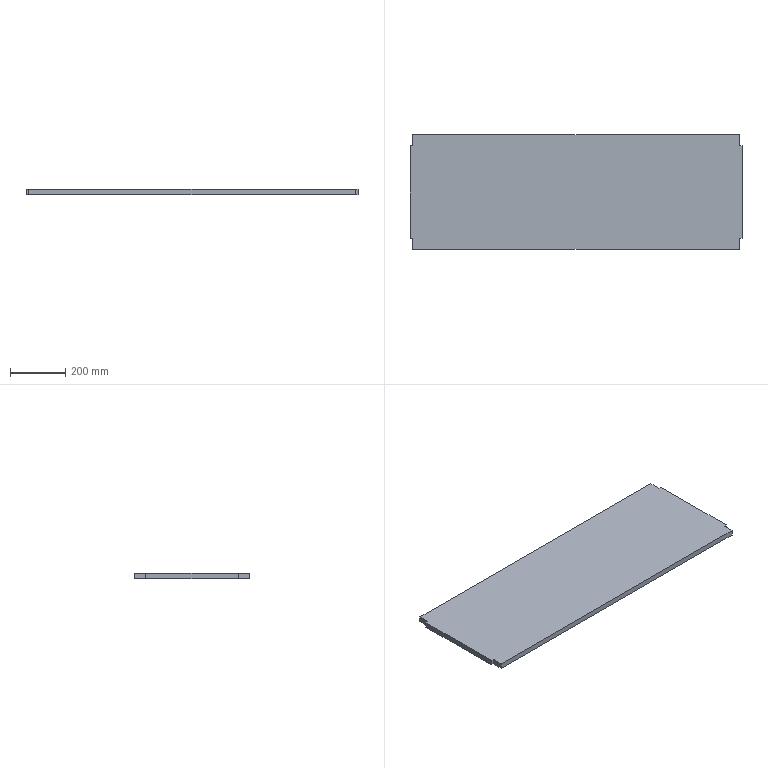Part | SolidWorks | features Extrusion 1, ICE 1 | 1 solid | 14 faces | box 1200 x 415 x 20 mm | volume 9928000 mm3 | plane 14
STEP:
#1=CARTESIAN_POINT('',(0.,375.,0.));
#2=VERTEX_POINT('',#1);
#3=CARTESIAN_POINT('',(0.,40.,0.));
#4=VERTEX_POINT('',#3);
#5=CARTESIAN_POINT('',(0.,0.,0.));
#6=DIRECTION('',(0.,-1.,0.));
#7=VECTOR('',#6,1000.);
#8=LINE('',#5,#7);
#9=EDGE_CURVE('',#2,#4,#8,.T.);
#10=ORIENTED_EDGE('',*,*,#9,.T.);
#11=CARTESIAN_POINT('',(0.,40.,20.));
#12=VERTEX_POINT('',#11);
#13=CARTESIAN_POINT('',(0.,40.,-260.));
#14=DIRECTION('',(0.,0.,1.));
#15=VECTOR('',#14,1000.);
#16=LINE('',#13,#15);
#17=EDGE_CURVE('',#4,#12,#16,.T.);
#18=ORIENTED_EDGE('',*,*,#17,.T.);
#19=CARTESIAN_POINT('',(0.,375.,20.));
#20=VERTEX_POINT('',#19);
#21=CARTESIAN_POINT('',(0.,0.,20.));
#22=DIRECTION('',(0.,-1.,0.));
#23=VECTOR('',#22,1000.);
#24=LINE('',#21,#23);
#25=EDGE_CURVE('',#20,#12,#24,.T.);
#26=ORIENTED_EDGE('',*,*,#25,.F.);
#27=CARTESIAN_POINT('',(0.,375.,-260.));
#28=DIRECTION('',(0.,0.,1.));
#29=VECTOR('',#28,1000.);
#30=LINE('',#27,#29);
#31=EDGE_CURVE('',#2,#20,#30,.T.);
#32=ORIENTED_EDGE('',*,*,#31,.F.);
#33=EDGE_LOOP('',(#10,#18,#26,#32));
#34=FACE_OUTER_BOUND('',#33,.T.);
#35=CARTESIAN_POINT('',(0.,0.,20.));
#36=DIRECTION('',(1.,0.,0.));
#37=DIRECTION('',(0.,0.,-1.));
#38=AXIS2_PLACEMENT_3D('',#35,#36,#37);
#39=PLANE('',#38);
#40=ADVANCED_FACE('',(#34),#39,.F.);
#41=CARTESIAN_POINT('',(10.,0.,20.));
#42=VERTEX_POINT('',#41);
#43=CARTESIAN_POINT('',(1190.,0.,20.));
#44=VERTEX_POINT('',#43);
#45=CARTESIAN_POINT('',(0.,0.,20.));
#46=DIRECTION('',(1.,0.,0.));
#47=VECTOR('',#46,1000.);
#48=LINE('',#45,#47);
#49=EDGE_CURVE('',#42,#44,#48,.T.);
#50=ORIENTED_EDGE('',*,*,#49,.F.);
#51=CARTESIAN_POINT('',(10.,0.,0.));
#52=VERTEX_POINT('',#51);
#53=CARTESIAN_POINT('',(10.,0.,-260.));
#54=DIRECTION('',(0.,0.,1.));
#55=VECTOR('',#54,1000.);
#56=LINE('',#53,#55);
#57=EDGE_CURVE('',#52,#42,#56,.T.);
#58=ORIENTED_EDGE('',*,*,#57,.F.);
#59=CARTESIAN_POINT('',(1190.,0.,0.));
#60=VERTEX_POINT('',#59);
#61=CARTESIAN_POINT('',(0.,0.,0.));
#62=DIRECTION('',(1.,0.,0.));
#63=VECTOR('',#62,1000.);
#64=LINE('',#61,#63);
#65=EDGE_CURVE('',#52,#60,#64,.T.);
#66=ORIENTED_EDGE('',*,*,#65,.T.);
#67=CARTESIAN_POINT('',(1190.,0.,-260.));
#68=DIRECTION('',(0.,0.,1.));
#69=VECTOR('',#68,1000.);
#70=LINE('',#67,#69);
#71=EDGE_CURVE('',#60,#44,#70,.T.);
#72=ORIENTED_EDGE('',*,*,#71,.T.);
#73=EDGE_LOOP('',(#50,#58,#66,#72));
#74=FACE_OUTER_BOUND('',#73,.T.);
#75=CARTESIAN_POINT('',(0.,0.,20.));
#76=DIRECTION('',(0.,1.,0.));
#77=DIRECTION('',(0.,0.,1.));
#78=AXIS2_PLACEMENT_3D('',#75,#76,#77);
#79=PLANE('',#78);
#80=ADVANCED_FACE('',(#74),#79,.F.);
#81=CARTESIAN_POINT('',(1200.,40.,20.));
#82=VERTEX_POINT('',#81);
#83=CARTESIAN_POINT('',(1200.,375.,20.));
#84=VERTEX_POINT('',#83);
#85=CARTESIAN_POINT('',(1200.,0.,20.));
#86=DIRECTION('',(0.,1.,0.));
#87=VECTOR('',#86,1000.);
#88=LINE('',#85,#87);
#89=EDGE_CURVE('',#82,#84,#88,.T.);
#90=ORIENTED_EDGE('',*,*,#89,.F.);
#91=CARTESIAN_POINT('',(1200.,40.,0.));
#92=VERTEX_POINT('',#91);
#93=CARTESIAN_POINT('',(1200.,40.,-260.));
#94=DIRECTION('',(0.,0.,1.));
#95=VECTOR('',#94,1000.);
#96=LINE('',#93,#95);
#97=EDGE_CURVE('',#92,#82,#96,.T.);
#98=ORIENTED_EDGE('',*,*,#97,.F.);
#99=CARTESIAN_POINT('',(1200.,375.,0.));
#100=VERTEX_POINT('',#99);
#101=CARTESIAN_POINT('',(1200.,0.,0.));
#102=DIRECTION('',(0.,1.,0.));
#103=VECTOR('',#102,1000.);
#104=LINE('',#101,#103);
#105=EDGE_CURVE('',#92,#100,#104,.T.);
#106=ORIENTED_EDGE('',*,*,#105,.T.);
#107=CARTESIAN_POINT('',(1200.,375.,-260.));
#108=DIRECTION('',(0.,0.,1.));
#109=VECTOR('',#108,1000.);
#110=LINE('',#107,#109);
#111=EDGE_CURVE('',#100,#84,#110,.T.);
#112=ORIENTED_EDGE('',*,*,#111,.T.);
#113=EDGE_LOOP('',(#90,#98,#106,#112));
#114=FACE_OUTER_BOUND('',#113,.T.);
#115=CARTESIAN_POINT('',(1200.,0.,20.));
#116=DIRECTION('',(-1.,0.,0.));
#117=DIRECTION('',(0.,0.,1.));
#118=AXIS2_PLACEMENT_3D('',#115,#116,#117);
#119=PLANE('',#118);
#120=ADVANCED_FACE('',(#114),#119,.F.);
#121=CARTESIAN_POINT('',(1190.,415.,20.));
#122=VERTEX_POINT('',#121);
#123=CARTESIAN_POINT('',(10.,415.,20.));
#124=VERTEX_POINT('',#123);
#125=CARTESIAN_POINT('',(0.,415.,20.));
#126=DIRECTION('',(-1.,0.,0.));
#127=VECTOR('',#126,1000.);
#128=LINE('',#125,#127);
#129=EDGE_CURVE('',#122,#124,#128,.T.);
#130=ORIENTED_EDGE('',*,*,#129,.F.);
#131=CARTESIAN_POINT('',(1190.,415.,0.));
#132=VERTEX_POINT('',#131);
#133=CARTESIAN_POINT('',(1190.,415.,-260.));
#134=DIRECTION('',(0.,0.,1.));
#135=VECTOR('',#134,1000.);
#136=LINE('',#133,#135);
#137=EDGE_CURVE('',#132,#122,#136,.T.);
#138=ORIENTED_EDGE('',*,*,#137,.F.);
#139=CARTESIAN_POINT('',(10.,415.,0.));
#140=VERTEX_POINT('',#139);
#141=CARTESIAN_POINT('',(0.,415.,0.));
#142=DIRECTION('',(-1.,0.,0.));
#143=VECTOR('',#142,1000.);
#144=LINE('',#141,#143);
#145=EDGE_CURVE('',#132,#140,#144,.T.);
#146=ORIENTED_EDGE('',*,*,#145,.T.);
#147=CARTESIAN_POINT('',(10.,415.,-260.));
#148=DIRECTION('',(0.,0.,1.));
#149=VECTOR('',#148,1000.);
#150=LINE('',#147,#149);
#151=EDGE_CURVE('',#140,#124,#150,.T.);
#152=ORIENTED_EDGE('',*,*,#151,.T.);
#153=EDGE_LOOP('',(#130,#138,#146,#152));
#154=FACE_OUTER_BOUND('',#153,.T.);
#155=CARTESIAN_POINT('',(0.,415.,20.));
#156=DIRECTION('',(0.,-1.,0.));
#157=DIRECTION('',(0.,0.,-1.));
#158=AXIS2_PLACEMENT_3D('',#155,#156,#157);
#159=PLANE('',#158);
#160=ADVANCED_FACE('',(#154),#159,.F.);
#161=ORIENTED_EDGE('',*,*,#25,.T.);
#162=CARTESIAN_POINT('',(10.,40.,20.));
#163=VERTEX_POINT('',#162);
#164=CARTESIAN_POINT('',(0.,40.,20.));
#165=DIRECTION('',(-1.,0.,0.));
#166=VECTOR('',#165,1000.);
#167=LINE('',#164,#166);
#168=EDGE_CURVE('',#163,#12,#167,.T.);
#169=ORIENTED_EDGE('',*,*,#168,.F.);
#170=CARTESIAN_POINT('',(10.,0.,20.));
#171=DIRECTION('',(0.,1.,0.));
#172=VECTOR('',#171,1000.);
#173=LINE('',#170,#172);
#174=EDGE_CURVE('',#42,#163,#173,.T.);
#175=ORIENTED_EDGE('',*,*,#174,.F.);
#176=ORIENTED_EDGE('',*,*,#49,.T.);
#177=CARTESIAN_POINT('',(1190.,40.,20.));
#178=VERTEX_POINT('',#177);
#179=CARTESIAN_POINT('',(1190.,0.,20.));
#180=DIRECTION('',(0.,-1.,0.));
#181=VECTOR('',#180,1000.);
#182=LINE('',#179,#181);
#183=EDGE_CURVE('',#178,#44,#182,.T.);
#184=ORIENTED_EDGE('',*,*,#183,.F.);
#185=CARTESIAN_POINT('',(1200.,40.,20.));
#186=DIRECTION('',(-1.,0.,0.));
#187=VECTOR('',#186,1000.);
#188=LINE('',#185,#187);
#189=EDGE_CURVE('',#82,#178,#188,.T.);
#190=ORIENTED_EDGE('',*,*,#189,.F.);
#191=ORIENTED_EDGE('',*,*,#89,.T.);
#192=CARTESIAN_POINT('',(1190.,375.,20.));
#193=VERTEX_POINT('',#192);
#194=CARTESIAN_POINT('',(1190.,375.,20.));
#195=DIRECTION('',(1.,0.,0.));
#196=VECTOR('',#195,1000.);
#197=LINE('',#194,#196);
#198=EDGE_CURVE('',#193,#84,#197,.T.);
#199=ORIENTED_EDGE('',*,*,#198,.F.);
#200=CARTESIAN_POINT('',(1190.,415.,20.));
#201=DIRECTION('',(0.,-1.,0.));
#202=VECTOR('',#201,1000.);
#203=LINE('',#200,#202);
#204=EDGE_CURVE('',#122,#193,#203,.T.);
#205=ORIENTED_EDGE('',*,*,#204,.F.);
#206=ORIENTED_EDGE('',*,*,#129,.T.);
#207=CARTESIAN_POINT('',(10.,375.,20.));
#208=VERTEX_POINT('',#207);
#209=CARTESIAN_POINT('',(10.,415.,20.));
#210=DIRECTION('',(0.,1.,0.));
#211=VECTOR('',#210,1000.);
#212=LINE('',#209,#211);
#213=EDGE_CURVE('',#208,#124,#212,.T.);
#214=ORIENTED_EDGE('',*,*,#213,.F.);
#215=CARTESIAN_POINT('',(0.,375.,20.));
#216=DIRECTION('',(1.,0.,0.));
#217=VECTOR('',#216,1000.);
#218=LINE('',#215,#217);
#219=EDGE_CURVE('',#20,#208,#218,.T.);
#220=ORIENTED_EDGE('',*,*,#219,.F.);
#221=EDGE_LOOP('',(#161,#169,#175,#176,#184,#190,#191,#199,#205,#206,#214,#220));
#222=FACE_OUTER_BOUND('',#221,.T.);
#223=CARTESIAN_POINT('',(0.,0.,20.));
#224=DIRECTION('',(0.,0.,-1.));
#225=DIRECTION('',(-1.,0.,0.));
#226=AXIS2_PLACEMENT_3D('',#223,#224,#225);
#227=PLANE('',#226);
#228=ADVANCED_FACE('',(#222),#227,.F.);
#229=CARTESIAN_POINT('',(10.,40.,0.));
#230=VERTEX_POINT('',#229);
#231=CARTESIAN_POINT('',(0.,40.,0.));
#232=DIRECTION('',(1.,0.,0.));
#233=VECTOR('',#232,1000.);
#234=LINE('',#231,#233);
#235=EDGE_CURVE('',#4,#230,#234,.T.);
#236=ORIENTED_EDGE('',*,*,#235,.F.);
#237=ORIENTED_EDGE('',*,*,#9,.F.);
#238=CARTESIAN_POINT('',(10.,375.,0.));
#239=VERTEX_POINT('',#238);
#240=CARTESIAN_POINT('',(0.,375.,0.));
#241=DIRECTION('',(-1.,0.,0.));
#242=VECTOR('',#241,1000.);
#243=LINE('',#240,#242);
#244=EDGE_CURVE('',#239,#2,#243,.T.);
#245=ORIENTED_EDGE('',*,*,#244,.F.);
#246=CARTESIAN_POINT('',(10.,0.,0.));
#247=DIRECTION('',(0.,-1.,0.));
#248=VECTOR('',#247,1000.);
#249=LINE('',#246,#248);
#250=EDGE_CURVE('',#140,#239,#249,.T.);
#251=ORIENTED_EDGE('',*,*,#250,.F.);
#252=ORIENTED_EDGE('',*,*,#145,.F.);
#253=CARTESIAN_POINT('',(1190.,375.,0.));
#254=VERTEX_POINT('',#253);
#255=CARTESIAN_POINT('',(1190.,0.,0.));
#256=DIRECTION('',(0.,1.,0.));
#257=VECTOR('',#256,1000.);
#258=LINE('',#255,#257);
#259=EDGE_CURVE('',#254,#132,#258,.T.);
#260=ORIENTED_EDGE('',*,*,#259,.F.);
#261=CARTESIAN_POINT('',(0.,375.,0.));
#262=DIRECTION('',(-1.,0.,0.));
#263=VECTOR('',#262,1000.);
#264=LINE('',#261,#263);
#265=EDGE_CURVE('',#100,#254,#264,.T.);
#266=ORIENTED_EDGE('',*,*,#265,.F.);
#267=ORIENTED_EDGE('',*,*,#105,.F.);
#268=CARTESIAN_POINT('',(1190.,40.,0.));
#269=VERTEX_POINT('',#268);
#270=CARTESIAN_POINT('',(0.,40.,0.));
#271=DIRECTION('',(1.,0.,0.));
#272=VECTOR('',#271,1000.);
#273=LINE('',#270,#272);
#274=EDGE_CURVE('',#269,#92,#273,.T.);
#275=ORIENTED_EDGE('',*,*,#274,.F.);
#276=CARTESIAN_POINT('',(1190.,0.,0.));
#277=DIRECTION('',(0.,1.,0.));
#278=VECTOR('',#277,1000.);
#279=LINE('',#276,#278);
#280=EDGE_CURVE('',#60,#269,#279,.T.);
#281=ORIENTED_EDGE('',*,*,#280,.F.);
#282=ORIENTED_EDGE('',*,*,#65,.F.);
#283=CARTESIAN_POINT('',(10.,0.,0.));
#284=DIRECTION('',(0.,-1.,0.));
#285=VECTOR('',#284,1000.);
#286=LINE('',#283,#285);
#287=EDGE_CURVE('',#230,#52,#286,.T.);
#288=ORIENTED_EDGE('',*,*,#287,.F.);
#289=EDGE_LOOP('',(#236,#237,#245,#251,#252,#260,#266,#267,#275,#281,#282,#288));
#290=FACE_OUTER_BOUND('',#289,.T.);
#291=CARTESIAN_POINT('',(0.,0.,0.));
#292=DIRECTION('',(0.,0.,-1.));
#293=DIRECTION('',(-1.,0.,0.));
#294=AXIS2_PLACEMENT_3D('',#291,#292,#293);
#295=PLANE('',#294);
#296=ADVANCED_FACE('',(#290),#295,.T.);
#297=ORIENTED_EDGE('',*,*,#250,.T.);
#298=CARTESIAN_POINT('',(10.,375.,-260.));
#299=DIRECTION('',(0.,0.,1.));
#300=VECTOR('',#299,1000.);
#301=LINE('',#298,#300);
#302=EDGE_CURVE('',#239,#208,#301,.T.);
#303=ORIENTED_EDGE('',*,*,#302,.T.);
#304=ORIENTED_EDGE('',*,*,#213,.T.);
#305=ORIENTED_EDGE('',*,*,#151,.F.);
#306=EDGE_LOOP('',(#297,#303,#304,#305));
#307=FACE_OUTER_BOUND('',#306,.T.);
#308=CARTESIAN_POINT('',(10.,415.,-260.));
#309=DIRECTION('',(1.,0.,0.));
#310=DIRECTION('',(0.,1.,0.));
#311=AXIS2_PLACEMENT_3D('',#308,#309,#310);
#312=PLANE('',#311);
#313=ADVANCED_FACE('',(#307),#312,.F.);
#314=ORIENTED_EDGE('',*,*,#244,.T.);
#315=ORIENTED_EDGE('',*,*,#31,.T.);
#316=ORIENTED_EDGE('',*,*,#219,.T.);
#317=ORIENTED_EDGE('',*,*,#302,.F.);
#318=EDGE_LOOP('',(#314,#315,#316,#317));
#319=FACE_OUTER_BOUND('',#318,.T.);
#320=CARTESIAN_POINT('',(0.,375.,-260.));
#321=DIRECTION('',(0.,-1.,0.));
#322=DIRECTION('',(0.,0.,-1.));
#323=AXIS2_PLACEMENT_3D('',#320,#321,#322);
#324=PLANE('',#323);
#325=ADVANCED_FACE('',(#319),#324,.F.);
#326=ORIENTED_EDGE('',*,*,#259,.T.);
#327=ORIENTED_EDGE('',*,*,#137,.T.);
#328=ORIENTED_EDGE('',*,*,#204,.T.);
#329=CARTESIAN_POINT('',(1190.,375.,-260.));
#330=DIRECTION('',(0.,0.,1.));
#331=VECTOR('',#330,1000.);
#332=LINE('',#329,#331);
#333=EDGE_CURVE('',#254,#193,#332,.T.);
#334=ORIENTED_EDGE('',*,*,#333,.F.);
#335=EDGE_LOOP('',(#326,#327,#328,#334));
#336=FACE_OUTER_BOUND('',#335,.T.);
#337=CARTESIAN_POINT('',(1190.,415.,-260.));
#338=DIRECTION('',(-1.,0.,0.));
#339=DIRECTION('',(0.,0.,1.));
#340=AXIS2_PLACEMENT_3D('',#337,#338,#339);
#341=PLANE('',#340);
#342=ADVANCED_FACE('',(#336),#341,.F.);
#343=ORIENTED_EDGE('',*,*,#265,.T.);
#344=ORIENTED_EDGE('',*,*,#333,.T.);
#345=ORIENTED_EDGE('',*,*,#198,.T.);
#346=ORIENTED_EDGE('',*,*,#111,.F.);
#347=EDGE_LOOP('',(#343,#344,#345,#346));
#348=FACE_OUTER_BOUND('',#347,.T.);
#349=CARTESIAN_POINT('',(1190.,375.,-260.));
#350=DIRECTION('',(0.,-1.,0.));
#351=DIRECTION('',(0.,0.,-1.));
#352=AXIS2_PLACEMENT_3D('',#349,#350,#351);
#353=PLANE('',#352);
#354=ADVANCED_FACE('',(#348),#353,.F.);
#355=ORIENTED_EDGE('',*,*,#280,.T.);
#356=CARTESIAN_POINT('',(1190.,40.,-260.));
#357=DIRECTION('',(0.,0.,1.));
#358=VECTOR('',#357,1000.);
#359=LINE('',#356,#358);
#360=EDGE_CURVE('',#269,#178,#359,.T.);
#361=ORIENTED_EDGE('',*,*,#360,.T.);
#362=ORIENTED_EDGE('',*,*,#183,.T.);
#363=ORIENTED_EDGE('',*,*,#71,.F.);
#364=EDGE_LOOP('',(#355,#361,#362,#363));
#365=FACE_OUTER_BOUND('',#364,.T.);
#366=CARTESIAN_POINT('',(1190.,0.,-260.));
#367=DIRECTION('',(-1.,0.,0.));
#368=DIRECTION('',(0.,0.,1.));
#369=AXIS2_PLACEMENT_3D('',#366,#367,#368);
#370=PLANE('',#369);
#371=ADVANCED_FACE('',(#365),#370,.F.);
#372=ORIENTED_EDGE('',*,*,#274,.T.);
#373=ORIENTED_EDGE('',*,*,#97,.T.);
#374=ORIENTED_EDGE('',*,*,#189,.T.);
#375=ORIENTED_EDGE('',*,*,#360,.F.);
#376=EDGE_LOOP('',(#372,#373,#374,#375));
#377=FACE_OUTER_BOUND('',#376,.T.);
#378=CARTESIAN_POINT('',(1200.,40.,-260.));
#379=DIRECTION('',(0.,1.,0.));
#380=DIRECTION('',(-1.,0.,0.));
#381=AXIS2_PLACEMENT_3D('',#378,#379,#380);
#382=PLANE('',#381);
#383=ADVANCED_FACE('',(#377),#382,.F.);
#384=ORIENTED_EDGE('',*,*,#235,.T.);
#385=CARTESIAN_POINT('',(10.,40.,-260.));
#386=DIRECTION('',(0.,0.,1.));
#387=VECTOR('',#386,1000.);
#388=LINE('',#385,#387);
#389=EDGE_CURVE('',#230,#163,#388,.T.);
#390=ORIENTED_EDGE('',*,*,#389,.T.);
#391=ORIENTED_EDGE('',*,*,#168,.T.);
#392=ORIENTED_EDGE('',*,*,#17,.F.);
#393=EDGE_LOOP('',(#384,#390,#391,#392));
#394=FACE_OUTER_BOUND('',#393,.T.);
#395=CARTESIAN_POINT('',(0.,40.,-260.));
#396=DIRECTION('',(0.,1.,0.));
#397=DIRECTION('',(0.,0.,1.));
#398=AXIS2_PLACEMENT_3D('',#395,#396,#397);
#399=PLANE('',#398);
#400=ADVANCED_FACE('',(#394),#399,.F.);
#401=ORIENTED_EDGE('',*,*,#287,.T.);
#402=ORIENTED_EDGE('',*,*,#57,.T.);
#403=ORIENTED_EDGE('',*,*,#174,.T.);
#404=ORIENTED_EDGE('',*,*,#389,.F.);
#405=EDGE_LOOP('',(#401,#402,#403,#404));
#406=FACE_OUTER_BOUND('',#405,.T.);
#407=CARTESIAN_POINT('',(10.,0.,-260.));
#408=DIRECTION('',(1.,0.,0.));
#409=DIRECTION('',(0.,0.,-1.));
#410=AXIS2_PLACEMENT_3D('',#407,#408,#409);
#411=PLANE('',#410);
#412=ADVANCED_FACE('',(#406),#411,.F.);
#413=CLOSED_SHELL('',(#40,#80,#120,#160,#228,#296,#313,#325,#342,#354,#371,#383,#400,#412));
#414=MANIFOLD_SOLID_BREP('',#413);
#415=CARTESIAN_POINT('',(0.,0.,0.));
#416=DIRECTION('',(0.,0.,1.));
#417=DIRECTION('',(1.,0.,0.));
#418=AXIS2_PLACEMENT_3D('',#415,#416,#417);
#419=(LENGTH_UNIT()NAMED_UNIT(*)SI_UNIT(.MILLI.,.METRE.));
#420=UNCERTAINTY_MEASURE_WITH_UNIT(LENGTH_MEASURE(0.00001),#419,'','');
#421=(NAMED_UNIT(*)PLANE_ANGLE_UNIT()SI_UNIT($,.RADIAN.));
#422=(NAMED_UNIT(*)SI_UNIT($,.STERADIAN.)SOLID_ANGLE_UNIT());
#423=(GEOMETRIC_REPRESENTATION_CONTEXT(3)GLOBAL_UNCERTAINTY_ASSIGNED_CONTEXT((#420))GLOBAL_UNIT_ASSIGNED_CONTEXT((#419,#421,#422))REPRESENTATION_CONTEXT('',''));
#424=ADVANCED_BREP_SHAPE_REPRESENTATION('',(#414,#418),#423);